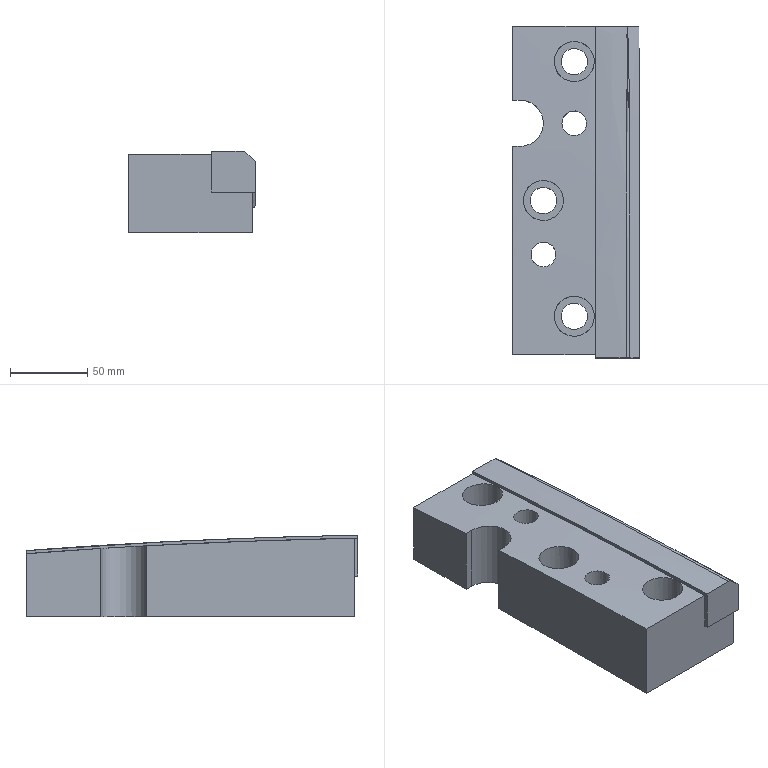Part | NX | features MAIN_BODY 2 | 1 solid | 31 faces | box 82.244 x 215 x 53.064 mm | volume 725143 mm3 | plane 14 | cylinder 9 | spline 8 | commonest cylinder face diameters 17 x3 26 x3 16 x2 30 x1